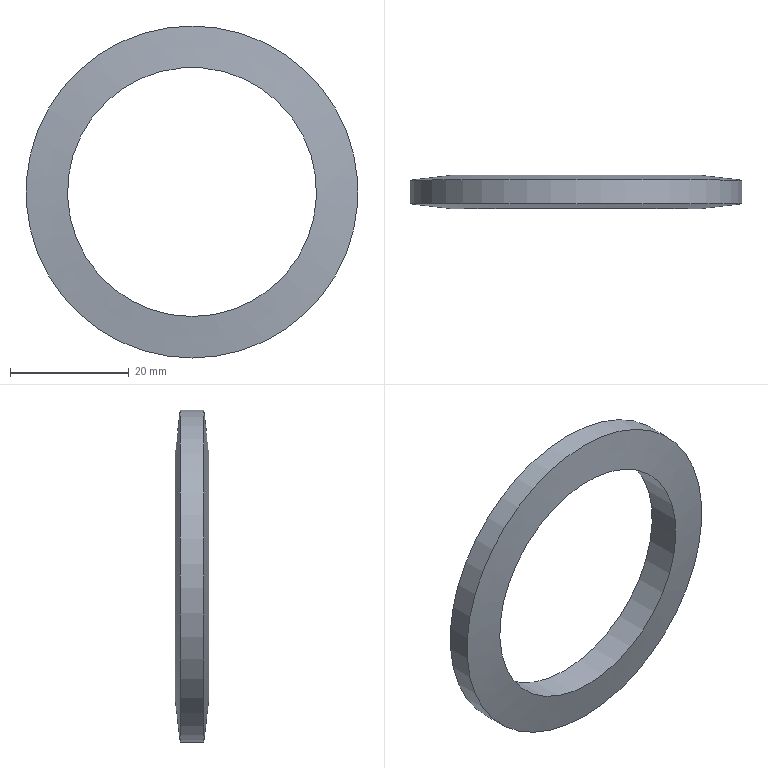Part | NX | features DATUM_CSYS 2, SKETCH 1, SWP104 1 | 1 solid | 4 faces | box 56 x 5.63 x 56 mm | volume 5147 mm3 | cone 2 | cylinder 2 | commonest cylinder face diameters 42 x1 56 x1
STEP:
#1=CARTESIAN_POINT('',(0.,-2.815,-21.));
#2=VERTEX_POINT('',#1);
#3=CARTESIAN_POINT('',(0.,-2.815,0.));
#4=DIRECTION('',(0.,-1.,0.));
#5=DIRECTION('',(0.,0.,-1.));
#6=AXIS2_PLACEMENT_3D('',#3,#4,#5);
#7=CIRCLE('',#6,21.);
#8=EDGE_CURVE('',#2,#2,#7,.T.);
#9=ORIENTED_EDGE('',*,*,#8,.F.);
#10=EDGE_LOOP('',(#9));
#11=FACE_BOUND('',#10,.T.);
#12=CARTESIAN_POINT('',(0.,-2.,-28.));
#13=VERTEX_POINT('',#12);
#14=CARTESIAN_POINT('',(0.,-2.,0.));
#15=DIRECTION('',(0.,-1.,0.));
#16=DIRECTION('',(0.,0.,-1.));
#17=AXIS2_PLACEMENT_3D('',#14,#15,#16);
#18=CIRCLE('',#17,28.);
#19=EDGE_CURVE('',#13,#13,#18,.T.);
#20=ORIENTED_EDGE('',*,*,#19,.T.);
#21=EDGE_LOOP('',(#20));
#22=FACE_BOUND('',#21,.T.);
#23=CARTESIAN_POINT('',(0.,-2.,0.));
#24=DIRECTION('',(0.,1.,0.));
#25=DIRECTION('',(0.,0.,1.));
#26=AXIS2_PLACEMENT_3D('',#23,#24,#25);
#27=CONICAL_SURFACE('',#26,28.,1.455);
#28=ADVANCED_FACE('',(#11,#22),#27,.T.);
#29=CARTESIAN_POINT('',(0.,2.815,-21.));
#30=VERTEX_POINT('',#29);
#31=CARTESIAN_POINT('',(0.,2.815,0.));
#32=DIRECTION('',(0.,-1.,0.));
#33=DIRECTION('',(0.,0.,-1.));
#34=AXIS2_PLACEMENT_3D('',#31,#32,#33);
#35=CIRCLE('',#34,21.);
#36=EDGE_CURVE('',#30,#30,#35,.T.);
#37=ORIENTED_EDGE('',*,*,#36,.F.);
#38=EDGE_LOOP('',(#37));
#39=FACE_BOUND('',#38,.T.);
#40=ORIENTED_EDGE('',*,*,#8,.T.);
#41=EDGE_LOOP('',(#40));
#42=FACE_BOUND('',#41,.T.);
#43=CARTESIAN_POINT('',(0.,0.,0.));
#44=DIRECTION('',(0.,-1.,0.));
#45=DIRECTION('',(0.,0.,-1.));
#46=AXIS2_PLACEMENT_3D('',#43,#44,#45);
#47=CYLINDRICAL_SURFACE('',#46,21.);
#48=ADVANCED_FACE('',(#39,#42),#47,.F.);
#49=CARTESIAN_POINT('',(0.,2.,-28.));
#50=VERTEX_POINT('',#49);
#51=CARTESIAN_POINT('',(0.,2.,0.));
#52=DIRECTION('',(0.,-1.,0.));
#53=DIRECTION('',(0.,0.,-1.));
#54=AXIS2_PLACEMENT_3D('',#51,#52,#53);
#55=CIRCLE('',#54,28.);
#56=EDGE_CURVE('',#50,#50,#55,.T.);
#57=ORIENTED_EDGE('',*,*,#56,.F.);
#58=EDGE_LOOP('',(#57));
#59=FACE_BOUND('',#58,.T.);
#60=ORIENTED_EDGE('',*,*,#36,.T.);
#61=EDGE_LOOP('',(#60));
#62=FACE_BOUND('',#61,.T.);
#63=CARTESIAN_POINT('',(0.,2.815,0.));
#64=DIRECTION('',(0.,-1.,0.));
#65=DIRECTION('',(0.,0.,-1.));
#66=AXIS2_PLACEMENT_3D('',#63,#64,#65);
#67=CONICAL_SURFACE('',#66,21.,1.455);
#68=ADVANCED_FACE('',(#59,#62),#67,.T.);
#69=ORIENTED_EDGE('',*,*,#19,.F.);
#70=EDGE_LOOP('',(#69));
#71=FACE_BOUND('',#70,.T.);
#72=ORIENTED_EDGE('',*,*,#56,.T.);
#73=EDGE_LOOP('',(#72));
#74=FACE_BOUND('',#73,.T.);
#75=CARTESIAN_POINT('',(0.,0.,0.));
#76=DIRECTION('',(0.,-1.,0.));
#77=DIRECTION('',(0.,0.,-1.));
#78=AXIS2_PLACEMENT_3D('',#75,#76,#77);
#79=CYLINDRICAL_SURFACE('',#78,28.);
#80=ADVANCED_FACE('',(#71,#74),#79,.T.);
#81=CLOSED_SHELL('',(#28,#48,#68,#80));
#82=MANIFOLD_SOLID_BREP('',#81);
#83=(LENGTH_UNIT()NAMED_UNIT(*)SI_UNIT(.MILLI.,.METRE.));
#84=UNCERTAINTY_MEASURE_WITH_UNIT(LENGTH_MEASURE(0.00001),#83,'','');
#85=(NAMED_UNIT(*)PLANE_ANGLE_UNIT()SI_UNIT($,.RADIAN.));
#86=(NAMED_UNIT(*)SI_UNIT($,.STERADIAN.)SOLID_ANGLE_UNIT());
#87=(GEOMETRIC_REPRESENTATION_CONTEXT(3)GLOBAL_UNCERTAINTY_ASSIGNED_CONTEXT((#84))GLOBAL_UNIT_ASSIGNED_CONTEXT((#83,#85,#86))REPRESENTATION_CONTEXT('',''));
#88=ADVANCED_BREP_SHAPE_REPRESENTATION('',(#82),#87);